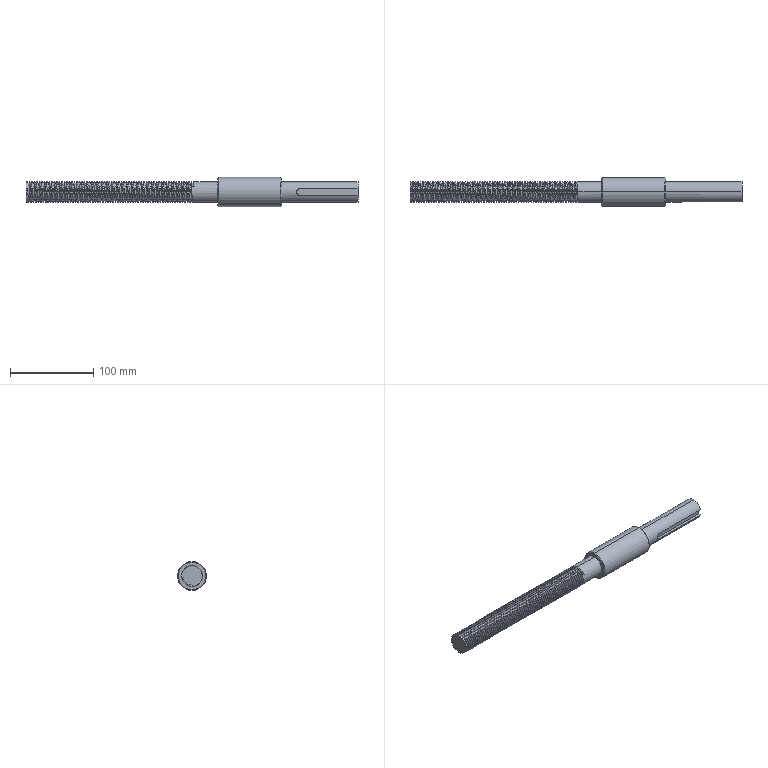Part | SolidWorks | features ICE 3, Chamfer 1, Extrusion 1, HoleWzd 1, SweepThread 1 | 1 solid | 162 faces | box 400 x 35 x 35 mm | volume 215314 mm3 | cylinder 142 | plane 9 | cone 8 | spline 3 | commonest cylinder face diameters 25 x137 8.5 x2 35 x2 8 x1